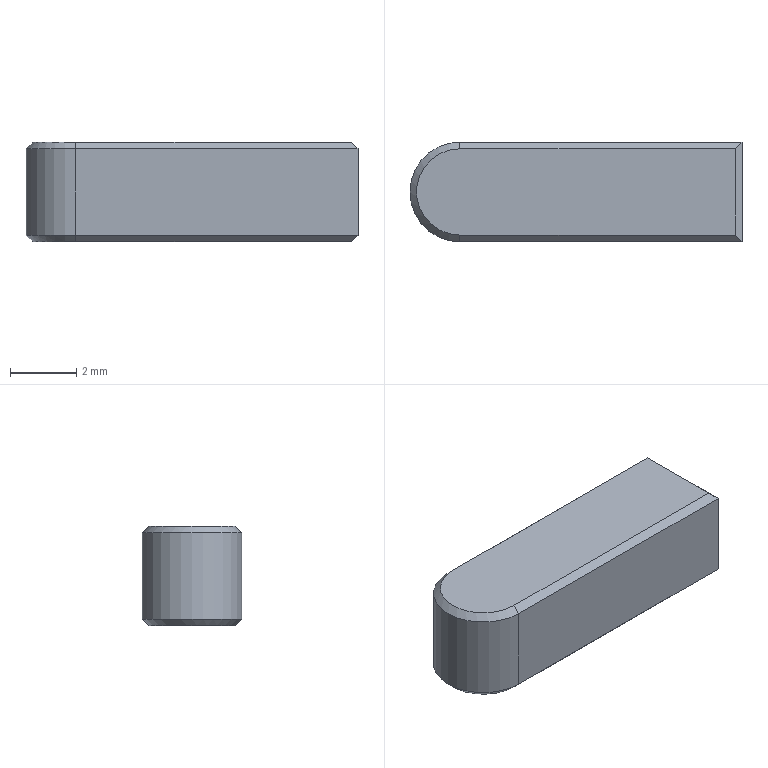Part | NX | features BREP 1, DATUM_CSYS 1 | 1 solid | 14 faces | box 10 x 3 x 3 mm | volume 86.133 mm3 | plane 11 | cone 2 | cylinder 1 | commonest cylinder face diameters 3 x1
STEP:
#1=CARTESIAN_POINT('',(-3.5,1.3,0.));
#2=VERTEX_POINT('',#1);
#3=CARTESIAN_POINT('',(-3.5,-1.3,0.));
#4=VERTEX_POINT('',#3);
#5=CARTESIAN_POINT('',(-3.5,0.,0.));
#6=DIRECTION('',(0.,0.,1.));
#7=DIRECTION('',(0.,1.,0.));
#8=AXIS2_PLACEMENT_3D('',#5,#6,#7);
#9=CIRCLE('',#8,1.3);
#10=EDGE_CURVE('',#2,#4,#9,.T.);
#11=ORIENTED_EDGE('',*,*,#10,.F.);
#12=CARTESIAN_POINT('',(4.8,1.3,0.));
#13=VERTEX_POINT('',#12);
#14=CARTESIAN_POINT('',(4.8,1.3,0.));
#15=DIRECTION('',(-1.,0.,0.));
#16=VECTOR('',#15,1000.);
#17=LINE('',#14,#16);
#18=EDGE_CURVE('',#13,#2,#17,.T.);
#19=ORIENTED_EDGE('',*,*,#18,.F.);
#20=CARTESIAN_POINT('',(4.8,-1.3,0.));
#21=VERTEX_POINT('',#20);
#22=CARTESIAN_POINT('',(4.8,-1.3,0.));
#23=DIRECTION('',(0.,1.,0.));
#24=VECTOR('',#23,1000.);
#25=LINE('',#22,#24);
#26=EDGE_CURVE('',#21,#13,#25,.T.);
#27=ORIENTED_EDGE('',*,*,#26,.F.);
#28=CARTESIAN_POINT('',(-3.5,-1.3,0.));
#29=DIRECTION('',(1.,0.,0.));
#30=VECTOR('',#29,1000.);
#31=LINE('',#28,#30);
#32=EDGE_CURVE('',#4,#21,#31,.T.);
#33=ORIENTED_EDGE('',*,*,#32,.F.);
#34=EDGE_LOOP('',(#11,#19,#27,#33));
#35=FACE_BOUND('',#34,.T.);
#36=CARTESIAN_POINT('',(0.,3.5,0.));
#37=DIRECTION('',(0.,0.,1.));
#38=DIRECTION('',(-1.,0.,0.));
#39=AXIS2_PLACEMENT_3D('',#36,#37,#38);
#40=PLANE('',#39);
#41=ADVANCED_FACE('',(#35),#40,.F.);
#42=CARTESIAN_POINT('',(-3.5,-1.3,3.));
#43=VERTEX_POINT('',#42);
#44=CARTESIAN_POINT('',(4.8,-1.3,3.));
#45=VERTEX_POINT('',#44);
#46=CARTESIAN_POINT('',(-3.5,-1.3,3.));
#47=DIRECTION('',(1.,0.,0.));
#48=VECTOR('',#47,1000.);
#49=LINE('',#46,#48);
#50=EDGE_CURVE('',#43,#45,#49,.T.);
#51=ORIENTED_EDGE('',*,*,#50,.T.);
#52=CARTESIAN_POINT('',(4.8,1.3,3.));
#53=VERTEX_POINT('',#52);
#54=CARTESIAN_POINT('',(4.8,-1.3,3.));
#55=DIRECTION('',(0.,1.,0.));
#56=VECTOR('',#55,1000.);
#57=LINE('',#54,#56);
#58=EDGE_CURVE('',#45,#53,#57,.T.);
#59=ORIENTED_EDGE('',*,*,#58,.T.);
#60=CARTESIAN_POINT('',(-3.5,1.3,3.));
#61=VERTEX_POINT('',#60);
#62=CARTESIAN_POINT('',(4.8,1.3,3.));
#63=DIRECTION('',(-1.,0.,0.));
#64=VECTOR('',#63,1000.);
#65=LINE('',#62,#64);
#66=EDGE_CURVE('',#53,#61,#65,.T.);
#67=ORIENTED_EDGE('',*,*,#66,.T.);
#68=CARTESIAN_POINT('',(-3.5,0.,3.));
#69=DIRECTION('',(0.,0.,1.));
#70=DIRECTION('',(0.,1.,0.));
#71=AXIS2_PLACEMENT_3D('',#68,#69,#70);
#72=CIRCLE('',#71,1.3);
#73=EDGE_CURVE('',#61,#43,#72,.T.);
#74=ORIENTED_EDGE('',*,*,#73,.T.);
#75=EDGE_LOOP('',(#51,#59,#67,#74));
#76=FACE_BOUND('',#75,.T.);
#77=CARTESIAN_POINT('',(0.,3.5,3.));
#78=DIRECTION('',(0.,0.,1.));
#79=DIRECTION('',(-1.,0.,0.));
#80=AXIS2_PLACEMENT_3D('',#77,#78,#79);
#81=PLANE('',#80);
#82=ADVANCED_FACE('',(#76),#81,.T.);
#83=CARTESIAN_POINT('',(5.,1.5,0.2));
#84=VERTEX_POINT('',#83);
#85=CARTESIAN_POINT('',(5.,1.5,2.8));
#86=VERTEX_POINT('',#85);
#87=CARTESIAN_POINT('',(5.,1.5,0.2));
#88=DIRECTION('',(0.,0.,1.));
#89=VECTOR('',#88,1000.);
#90=LINE('',#87,#89);
#91=EDGE_CURVE('',#84,#86,#90,.T.);
#92=ORIENTED_EDGE('',*,*,#91,.T.);
#93=CARTESIAN_POINT('',(5.,-1.5,2.8));
#94=VERTEX_POINT('',#93);
#95=CARTESIAN_POINT('',(5.,-1.5,2.8));
#96=DIRECTION('',(0.,1.,0.));
#97=VECTOR('',#96,1000.);
#98=LINE('',#95,#97);
#99=EDGE_CURVE('',#94,#86,#98,.T.);
#100=ORIENTED_EDGE('',*,*,#99,.F.);
#101=CARTESIAN_POINT('',(5.,-1.5,0.2));
#102=VERTEX_POINT('',#101);
#103=CARTESIAN_POINT('',(5.,-1.5,0.2));
#104=DIRECTION('',(0.,0.,1.));
#105=VECTOR('',#104,1000.);
#106=LINE('',#103,#105);
#107=EDGE_CURVE('',#102,#94,#106,.T.);
#108=ORIENTED_EDGE('',*,*,#107,.F.);
#109=CARTESIAN_POINT('',(5.,-1.5,0.2));
#110=DIRECTION('',(0.,1.,0.));
#111=VECTOR('',#110,1000.);
#112=LINE('',#109,#111);
#113=EDGE_CURVE('',#102,#84,#112,.T.);
#114=ORIENTED_EDGE('',*,*,#113,.T.);
#115=EDGE_LOOP('',(#92,#100,#108,#114));
#116=FACE_BOUND('',#115,.T.);
#117=CARTESIAN_POINT('',(5.,0.,1.5));
#118=DIRECTION('',(1.,0.,0.));
#119=DIRECTION('',(0.,-1.,0.));
#120=AXIS2_PLACEMENT_3D('',#117,#118,#119);
#121=PLANE('',#120);
#122=ADVANCED_FACE('',(#116),#121,.T.);
#123=ORIENTED_EDGE('',*,*,#91,.F.);
#124=CARTESIAN_POINT('',(-3.5,1.5,0.2));
#125=VERTEX_POINT('',#124);
#126=CARTESIAN_POINT('',(5.,1.5,0.2));
#127=DIRECTION('',(-1.,0.,-0.000000017));
#128=VECTOR('',#127,1000.);
#129=LINE('',#126,#128);
#130=EDGE_CURVE('',#84,#125,#129,.T.);
#131=ORIENTED_EDGE('',*,*,#130,.T.);
#132=CARTESIAN_POINT('',(-3.5,1.5,2.8));
#133=VERTEX_POINT('',#132);
#134=CARTESIAN_POINT('',(-3.5,1.5,0.2));
#135=DIRECTION('',(0.,0.,1.));
#136=VECTOR('',#135,1000.);
#137=LINE('',#134,#136);
#138=EDGE_CURVE('',#125,#133,#137,.T.);
#139=ORIENTED_EDGE('',*,*,#138,.T.);
#140=CARTESIAN_POINT('',(5.,1.5,2.8));
#141=DIRECTION('',(-1.,0.,0.000000017));
#142=VECTOR('',#141,1000.);
#143=LINE('',#140,#142);
#144=EDGE_CURVE('',#86,#133,#143,.T.);
#145=ORIENTED_EDGE('',*,*,#144,.F.);
#146=EDGE_LOOP('',(#123,#131,#139,#145));
#147=FACE_BOUND('',#146,.T.);
#148=CARTESIAN_POINT('',(0.75,1.5,1.5));
#149=DIRECTION('',(0.,1.,0.));
#150=DIRECTION('',(1.,0.,0.));
#151=AXIS2_PLACEMENT_3D('',#148,#149,#150);
#152=PLANE('',#151);
#153=ADVANCED_FACE('',(#147),#152,.T.);
#154=ORIENTED_EDGE('',*,*,#138,.F.);
#155=CARTESIAN_POINT('',(-3.5,-1.5,0.2));
#156=VERTEX_POINT('',#155);
#157=CARTESIAN_POINT('',(-3.5,0.,0.2));
#158=DIRECTION('',(0.000000099,0.,1.));
#159=DIRECTION('',(0.,1.,0.));
#160=AXIS2_PLACEMENT_3D('',#157,#158,#159);
#161=CIRCLE('',#160,1.5);
#162=EDGE_CURVE('',#125,#156,#161,.T.);
#163=ORIENTED_EDGE('',*,*,#162,.T.);
#164=CARTESIAN_POINT('',(-3.5,-1.5,2.8));
#165=VERTEX_POINT('',#164);
#166=CARTESIAN_POINT('',(-3.5,-1.5,0.2));
#167=DIRECTION('',(0.,0.,1.));
#168=VECTOR('',#167,1000.);
#169=LINE('',#166,#168);
#170=EDGE_CURVE('',#156,#165,#169,.T.);
#171=ORIENTED_EDGE('',*,*,#170,.T.);
#172=CARTESIAN_POINT('',(-3.5,0.,2.8));
#173=DIRECTION('',(-0.000000099,0.,1.));
#174=DIRECTION('',(0.,1.,0.));
#175=AXIS2_PLACEMENT_3D('',#172,#173,#174);
#176=CIRCLE('',#175,1.5);
#177=EDGE_CURVE('',#133,#165,#176,.T.);
#178=ORIENTED_EDGE('',*,*,#177,.F.);
#179=EDGE_LOOP('',(#154,#163,#171,#178));
#180=FACE_BOUND('',#179,.T.);
#181=CARTESIAN_POINT('',(-3.5,0.,0.));
#182=DIRECTION('',(0.,0.,1.));
#183=DIRECTION('',(0.,-1.,0.));
#184=AXIS2_PLACEMENT_3D('',#181,#182,#183);
#185=CYLINDRICAL_SURFACE('',#184,1.5);
#186=ADVANCED_FACE('',(#180),#185,.T.);
#187=ORIENTED_EDGE('',*,*,#107,.T.);
#188=CARTESIAN_POINT('',(-3.5,-1.5,2.8));
#189=DIRECTION('',(1.,0.,0.));
#190=VECTOR('',#189,1000.);
#191=LINE('',#188,#190);
#192=EDGE_CURVE('',#165,#94,#191,.T.);
#193=ORIENTED_EDGE('',*,*,#192,.F.);
#194=ORIENTED_EDGE('',*,*,#170,.F.);
#195=CARTESIAN_POINT('',(-3.5,-1.5,0.2));
#196=DIRECTION('',(1.,0.,0.));
#197=VECTOR('',#196,1000.);
#198=LINE('',#195,#197);
#199=EDGE_CURVE('',#156,#102,#198,.T.);
#200=ORIENTED_EDGE('',*,*,#199,.T.);
#201=EDGE_LOOP('',(#187,#193,#194,#200));
#202=FACE_BOUND('',#201,.T.);
#203=CARTESIAN_POINT('',(0.75,-1.5,1.5));
#204=DIRECTION('',(0.,-1.,0.));
#205=DIRECTION('',(-1.,0.,0.));
#206=AXIS2_PLACEMENT_3D('',#203,#204,#205);
#207=PLANE('',#206);
#208=ADVANCED_FACE('',(#202),#207,.T.);
#209=ORIENTED_EDGE('',*,*,#10,.T.);
#210=CARTESIAN_POINT('',(-3.5,-1.3,0.));
#211=DIRECTION('',(0.,-0.7071,0.7071));
#212=VECTOR('',#211,1000.);
#213=LINE('',#210,#212);
#214=EDGE_CURVE('',#4,#156,#213,.T.);
#215=ORIENTED_EDGE('',*,*,#214,.T.);
#216=ORIENTED_EDGE('',*,*,#162,.F.);
#217=CARTESIAN_POINT('',(-3.5,1.3,0.));
#218=DIRECTION('',(0.,0.7071,0.7071));
#219=VECTOR('',#218,1000.);
#220=LINE('',#217,#219);
#221=EDGE_CURVE('',#2,#125,#220,.T.);
#222=ORIENTED_EDGE('',*,*,#221,.F.);
#223=EDGE_LOOP('',(#209,#215,#216,#222));
#224=FACE_BOUND('',#223,.T.);
#225=CARTESIAN_POINT('',(-3.5,0.,0.));
#226=DIRECTION('',(0.,0.,1.));
#227=DIRECTION('',(0.,-1.,0.));
#228=AXIS2_PLACEMENT_3D('',#225,#226,#227);
#229=CONICAL_SURFACE('',#228,1.3,0.7854);
#230=ADVANCED_FACE('',(#224),#229,.T.);
#231=ORIENTED_EDGE('',*,*,#130,.F.);
#232=CARTESIAN_POINT('',(5.,1.5,0.2));
#233=DIRECTION('',(-0.5774,-0.5774,-0.5774));
#234=VECTOR('',#233,1000.);
#235=LINE('',#232,#234);
#236=EDGE_CURVE('',#84,#13,#235,.T.);
#237=ORIENTED_EDGE('',*,*,#236,.T.);
#238=ORIENTED_EDGE('',*,*,#18,.T.);
#239=ORIENTED_EDGE('',*,*,#221,.T.);
#240=EDGE_LOOP('',(#231,#237,#238,#239));
#241=FACE_BOUND('',#240,.T.);
#242=CARTESIAN_POINT('',(0.75,1.4,0.1));
#243=DIRECTION('',(0.,-0.7071,0.7071));
#244=DIRECTION('',(0.,-0.7071,-0.7071));
#245=AXIS2_PLACEMENT_3D('',#242,#243,#244);
#246=PLANE('',#245);
#247=ADVANCED_FACE('',(#241),#246,.F.);
#248=ORIENTED_EDGE('',*,*,#32,.T.);
#249=CARTESIAN_POINT('',(4.9,-1.4,0.1));
#250=DIRECTION('',(-0.5774,0.5774,-0.5774));
#251=VECTOR('',#250,1000.);
#252=LINE('',#249,#251);
#253=EDGE_CURVE('',#102,#21,#252,.T.);
#254=ORIENTED_EDGE('',*,*,#253,.F.);
#255=ORIENTED_EDGE('',*,*,#199,.F.);
#256=ORIENTED_EDGE('',*,*,#214,.F.);
#257=EDGE_LOOP('',(#248,#254,#255,#256));
#258=FACE_BOUND('',#257,.T.);
#259=CARTESIAN_POINT('',(0.75,-1.4,0.1));
#260=DIRECTION('',(0.,0.7071,0.7071));
#261=DIRECTION('',(0.,0.7071,-0.7071));
#262=AXIS2_PLACEMENT_3D('',#259,#260,#261);
#263=PLANE('',#262);
#264=ADVANCED_FACE('',(#258),#263,.F.);
#265=ORIENTED_EDGE('',*,*,#253,.T.);
#266=ORIENTED_EDGE('',*,*,#26,.T.);
#267=ORIENTED_EDGE('',*,*,#236,.F.);
#268=ORIENTED_EDGE('',*,*,#113,.F.);
#269=EDGE_LOOP('',(#265,#266,#267,#268));
#270=FACE_BOUND('',#269,.T.);
#271=CARTESIAN_POINT('',(4.9,0.,0.1));
#272=DIRECTION('',(-0.7071,0.,0.7071));
#273=DIRECTION('',(-0.7071,0.,-0.7071));
#274=AXIS2_PLACEMENT_3D('',#271,#272,#273);
#275=PLANE('',#274);
#276=ADVANCED_FACE('',(#270),#275,.F.);
#277=CARTESIAN_POINT('',(-3.5,1.3,3.));
#278=DIRECTION('',(0.,0.7071,-0.7071));
#279=VECTOR('',#278,1000.);
#280=LINE('',#277,#279);
#281=EDGE_CURVE('',#61,#133,#280,.T.);
#282=ORIENTED_EDGE('',*,*,#281,.T.);
#283=ORIENTED_EDGE('',*,*,#177,.T.);
#284=CARTESIAN_POINT('',(-3.5,-1.3,3.));
#285=DIRECTION('',(0.,-0.7071,-0.7071));
#286=VECTOR('',#285,1000.);
#287=LINE('',#284,#286);
#288=EDGE_CURVE('',#43,#165,#287,.T.);
#289=ORIENTED_EDGE('',*,*,#288,.F.);
#290=ORIENTED_EDGE('',*,*,#73,.F.);
#291=EDGE_LOOP('',(#282,#283,#289,#290));
#292=FACE_BOUND('',#291,.T.);
#293=CARTESIAN_POINT('',(-3.5,0.,3.));
#294=DIRECTION('',(0.,0.,-1.));
#295=DIRECTION('',(0.,-1.,0.));
#296=AXIS2_PLACEMENT_3D('',#293,#294,#295);
#297=CONICAL_SURFACE('',#296,1.3,0.7854);
#298=ADVANCED_FACE('',(#292),#297,.T.);
#299=ORIENTED_EDGE('',*,*,#281,.F.);
#300=ORIENTED_EDGE('',*,*,#66,.F.);
#301=CARTESIAN_POINT('',(5.,1.5,2.8));
#302=DIRECTION('',(-0.5774,-0.5774,0.5774));
#303=VECTOR('',#302,1000.);
#304=LINE('',#301,#303);
#305=EDGE_CURVE('',#86,#53,#304,.T.);
#306=ORIENTED_EDGE('',*,*,#305,.F.);
#307=ORIENTED_EDGE('',*,*,#144,.T.);
#308=EDGE_LOOP('',(#299,#300,#306,#307));
#309=FACE_BOUND('',#308,.T.);
#310=CARTESIAN_POINT('',(0.75,1.4,2.9));
#311=DIRECTION('',(0.,0.7071,0.7071));
#312=DIRECTION('',(0.,-0.7071,0.7071));
#313=AXIS2_PLACEMENT_3D('',#310,#311,#312);
#314=PLANE('',#313);
#315=ADVANCED_FACE('',(#309),#314,.T.);
#316=ORIENTED_EDGE('',*,*,#288,.T.);
#317=ORIENTED_EDGE('',*,*,#192,.T.);
#318=CARTESIAN_POINT('',(4.9,-1.4,2.9));
#319=DIRECTION('',(-0.5774,0.5774,0.5774));
#320=VECTOR('',#319,1000.);
#321=LINE('',#318,#320);
#322=EDGE_CURVE('',#94,#45,#321,.T.);
#323=ORIENTED_EDGE('',*,*,#322,.T.);
#324=ORIENTED_EDGE('',*,*,#50,.F.);
#325=EDGE_LOOP('',(#316,#317,#323,#324));
#326=FACE_BOUND('',#325,.T.);
#327=CARTESIAN_POINT('',(0.75,-1.4,2.9));
#328=DIRECTION('',(0.,-0.7071,0.7071));
#329=DIRECTION('',(0.,0.7071,0.7071));
#330=AXIS2_PLACEMENT_3D('',#327,#328,#329);
#331=PLANE('',#330);
#332=ADVANCED_FACE('',(#326),#331,.T.);
#333=ORIENTED_EDGE('',*,*,#99,.T.);
#334=ORIENTED_EDGE('',*,*,#305,.T.);
#335=ORIENTED_EDGE('',*,*,#58,.F.);
#336=ORIENTED_EDGE('',*,*,#322,.F.);
#337=EDGE_LOOP('',(#333,#334,#335,#336));
#338=FACE_BOUND('',#337,.T.);
#339=CARTESIAN_POINT('',(4.9,0.,2.9));
#340=DIRECTION('',(0.7071,0.,0.7071));
#341=DIRECTION('',(-0.7071,0.,0.7071));
#342=AXIS2_PLACEMENT_3D('',#339,#340,#341);
#343=PLANE('',#342);
#344=ADVANCED_FACE('',(#338),#343,.T.);
#345=CLOSED_SHELL('',(#41,#82,#122,#153,#186,#208,#230,#247,#264,#276,#298,#315,#332,#344));
#346=MANIFOLD_SOLID_BREP('',#345);
#347=(LENGTH_UNIT()NAMED_UNIT(*)SI_UNIT(.MILLI.,.METRE.));
#348=UNCERTAINTY_MEASURE_WITH_UNIT(LENGTH_MEASURE(0.00001),#347,'','');
#349=(NAMED_UNIT(*)PLANE_ANGLE_UNIT()SI_UNIT($,.RADIAN.));
#350=(NAMED_UNIT(*)SI_UNIT($,.STERADIAN.)SOLID_ANGLE_UNIT());
#351=(GEOMETRIC_REPRESENTATION_CONTEXT(3)GLOBAL_UNCERTAINTY_ASSIGNED_CONTEXT((#348))GLOBAL_UNIT_ASSIGNED_CONTEXT((#347,#349,#350))REPRESENTATION_CONTEXT('',''));
#352=ADVANCED_BREP_SHAPE_REPRESENTATION('',(#346),#351);